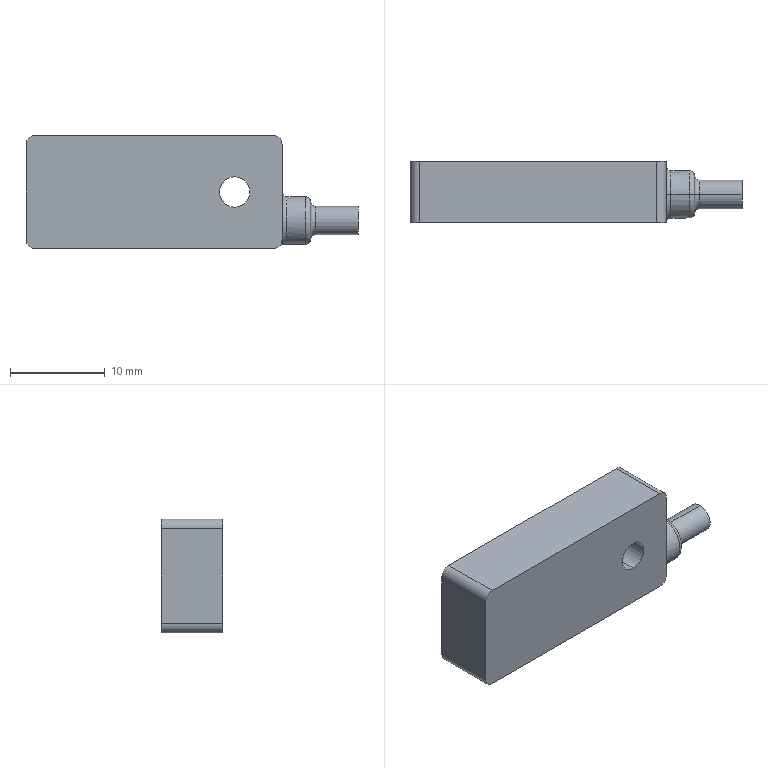Part | STEP file | APS4-12S-Z_Default | 1 solid | 88 faces | box 35 x 6.5 x 12 mm | volume 2071 mm3 | plane 49 | cylinder 32 | torus 6 | spline 1 | commonest cylinder face diameters 1.77 x6 0.183 x4 2 x4 2.015 x4 8 x4 3 x2